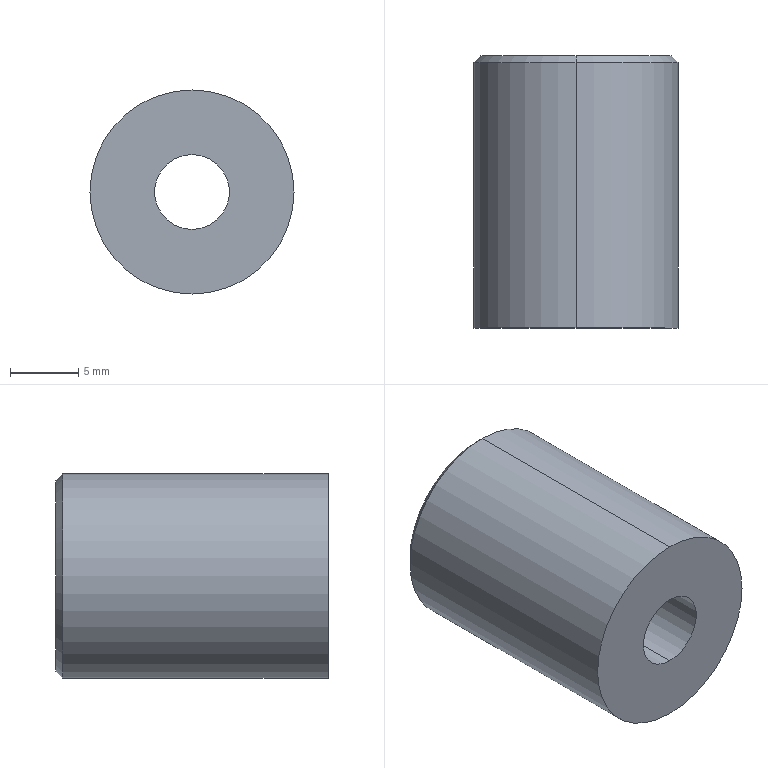Part | STEP file | PN_0011 | 1 solid | 11 faces | box 15 x 20 x 15 mm | volume 2655 mm3 | cylinder 6 | plane 3 | cone 2 | commonest cylinder face diameters 5.5 x2 9 x2 15 x2
STEP:
#1=CARTESIAN_POINT('',(0.,0.,0.));
#2=DIRECTION('',(0.,0.,1.));
#3=DIRECTION('',(1.,0.,0.));
#4=AXIS2_PLACEMENT_3D('',#1,#2,#3);
#5=CARTESIAN_POINT('',(0.,20.,7.));
#6=VERTEX_POINT('',#5);
#7=CARTESIAN_POINT('',(0.,20.,-7.));
#8=VERTEX_POINT('',#7);
#9=CARTESIAN_POINT('',(0.,20.,0.));
#10=DIRECTION('',(0.,1.,0.));
#11=DIRECTION('',(0.,0.,1.));
#12=AXIS2_PLACEMENT_3D('',#9,#10,#11);
#13=CIRCLE('',#12,7.);
#14=CARTESIAN_POINT('',(0.,20.,0.));
#15=DIRECTION('',(0.,-1.,0.));
#16=DIRECTION('',(0.,0.,-1.));
#17=AXIS2_PLACEMENT_3D('',#14,#15,#16);
#18=CONICAL_SURFACE('',#17,7.,0.7854);
#19=CARTESIAN_POINT('',(3.142,0.));
#20=DIRECTION('',(-1.,0.));
#21=VECTOR('',#20,1.);
#22=LINE('',#19,#21);
#23=(GEOMETRIC_REPRESENTATION_CONTEXT(2)PARAMETRIC_REPRESENTATION_CONTEXT()REPRESENTATION_CONTEXT('',''));
#24=DEFINITIONAL_REPRESENTATION('',(#22),#23);
#25=PCURVE('',#18,#24);
#26=CARTESIAN_POINT('',(0.,20.,0.));
#27=DIRECTION('',(0.,1.,0.));
#28=DIRECTION('',(0.,0.,1.));
#29=AXIS2_PLACEMENT_3D('',#26,#27,#28);
#30=PLANE('',#29);
#31=CARTESIAN_POINT('',(0.,0.));
#32=DIRECTION('',(1.,0.));
#33=AXIS2_PLACEMENT_2D('',#31,#32);
#34=CIRCLE('',#33,7.);
#35=(GEOMETRIC_REPRESENTATION_CONTEXT(2)PARAMETRIC_REPRESENTATION_CONTEXT()REPRESENTATION_CONTEXT('',''));
#36=DEFINITIONAL_REPRESENTATION('',(#34),#35);
#37=PCURVE('',#30,#36);
#38=SURFACE_CURVE('',#13,(#25,#37),.PCURVE_S1.);
#39=EDGE_CURVE('',#6,#8,#38,.T.);
#40=ORIENTED_EDGE('',*,*,#39,.F.);
#41=CARTESIAN_POINT('',(0.,19.5,7.5));
#42=VERTEX_POINT('',#41);
#43=CARTESIAN_POINT('',(0.,20.,7.));
#44=DIRECTION('',(0.,-0.7071,0.7071));
#45=VECTOR('',#44,1.);
#46=LINE('',#43,#45);
#47=CARTESIAN_POINT('',(3.142,0.));
#48=DIRECTION('',(0.,1.));
#49=VECTOR('',#48,1.);
#50=LINE('',#47,#49);
#51=(GEOMETRIC_REPRESENTATION_CONTEXT(2)PARAMETRIC_REPRESENTATION_CONTEXT()REPRESENTATION_CONTEXT('',''));
#52=DEFINITIONAL_REPRESENTATION('',(#50),#51);
#53=PCURVE('',#18,#52);
#54=CARTESIAN_POINT('',(0.,20.,0.));
#55=DIRECTION('',(0.,-1.,0.));
#56=DIRECTION('',(0.,0.,-1.));
#57=AXIS2_PLACEMENT_3D('',#54,#55,#56);
#58=CONICAL_SURFACE('',#57,7.,0.7854);
#59=CARTESIAN_POINT('',(3.142,0.));
#60=DIRECTION('',(0.,1.));
#61=VECTOR('',#60,1.);
#62=LINE('',#59,#61);
#63=(GEOMETRIC_REPRESENTATION_CONTEXT(2)PARAMETRIC_REPRESENTATION_CONTEXT()REPRESENTATION_CONTEXT('',''));
#64=DEFINITIONAL_REPRESENTATION('',(#62),#63);
#65=PCURVE('',#58,#64);
#66=SURFACE_CURVE('',#46,(#53,#65),.PCURVE_S1.);
#67=EDGE_CURVE('',#6,#42,#66,.T.);
#68=ORIENTED_EDGE('',*,*,#67,.T.);
#69=CARTESIAN_POINT('',(0.,19.5,-7.5));
#70=VERTEX_POINT('',#69);
#71=CARTESIAN_POINT('',(0.,19.5,0.));
#72=DIRECTION('',(0.,-1.,0.));
#73=DIRECTION('',(0.,0.,1.));
#74=AXIS2_PLACEMENT_3D('',#71,#72,#73);
#75=CIRCLE('',#74,7.5);
#76=CARTESIAN_POINT('',(-3.142,0.5));
#77=DIRECTION('',(1.,0.));
#78=VECTOR('',#77,1.);
#79=LINE('',#76,#78);
#80=(GEOMETRIC_REPRESENTATION_CONTEXT(2)PARAMETRIC_REPRESENTATION_CONTEXT()REPRESENTATION_CONTEXT('',''));
#81=DEFINITIONAL_REPRESENTATION('',(#79),#80);
#82=PCURVE('',#18,#81);
#83=CARTESIAN_POINT('',(0.,20.,0.));
#84=DIRECTION('',(0.,-1.,0.));
#85=DIRECTION('',(0.,0.,-1.));
#86=AXIS2_PLACEMENT_3D('',#83,#84,#85);
#87=CYLINDRICAL_SURFACE('',#86,7.5);
#88=CARTESIAN_POINT('',(-3.142,0.5));
#89=DIRECTION('',(1.,0.));
#90=VECTOR('',#89,1.);
#91=LINE('',#88,#90);
#92=(GEOMETRIC_REPRESENTATION_CONTEXT(2)PARAMETRIC_REPRESENTATION_CONTEXT()REPRESENTATION_CONTEXT('',''));
#93=DEFINITIONAL_REPRESENTATION('',(#91),#92);
#94=PCURVE('',#87,#93);
#95=SURFACE_CURVE('',#75,(#82,#94),.PCURVE_S1.);
#96=EDGE_CURVE('',#70,#42,#95,.T.);
#97=ORIENTED_EDGE('',*,*,#96,.F.);
#98=CARTESIAN_POINT('',(0.,20.,-7.));
#99=DIRECTION('',(0.,-0.7071,-0.7071));
#100=VECTOR('',#99,1.);
#101=LINE('',#98,#100);
#102=CARTESIAN_POINT('',(0.,0.));
#103=DIRECTION('',(0.,1.));
#104=VECTOR('',#103,1.);
#105=LINE('',#102,#104);
#106=(GEOMETRIC_REPRESENTATION_CONTEXT(2)PARAMETRIC_REPRESENTATION_CONTEXT()REPRESENTATION_CONTEXT('',''));
#107=DEFINITIONAL_REPRESENTATION('',(#105),#106);
#108=PCURVE('',#18,#107);
#109=CARTESIAN_POINT('',(6.283,0.));
#110=DIRECTION('',(0.,1.));
#111=VECTOR('',#110,1.);
#112=LINE('',#109,#111);
#113=(GEOMETRIC_REPRESENTATION_CONTEXT(2)PARAMETRIC_REPRESENTATION_CONTEXT()REPRESENTATION_CONTEXT('',''));
#114=DEFINITIONAL_REPRESENTATION('',(#112),#113);
#115=PCURVE('',#58,#114);
#116=SURFACE_CURVE('',#101,(#108,#115),.PCURVE_S1.);
#117=EDGE_CURVE('',#8,#70,#116,.T.);
#118=ORIENTED_EDGE('',*,*,#117,.F.);
#119=EDGE_LOOP('',(#40,#68,#97,#118));
#120=FACE_BOUND('',#119,.T.);
#121=ADVANCED_FACE('',(#120),#18,.T.);
#122=CARTESIAN_POINT('',(0.,10.,4.5));
#123=VERTEX_POINT('',#122);
#124=CARTESIAN_POINT('',(0.,20.,4.5));
#125=VERTEX_POINT('',#124);
#126=CARTESIAN_POINT('',(0.,20.,4.5));
#127=DIRECTION('',(0.,1.,0.));
#128=VECTOR('',#127,1.);
#129=LINE('',#126,#128);
#130=CARTESIAN_POINT('',(0.,20.,0.));
#131=DIRECTION('',(0.,1.,0.));
#132=DIRECTION('',(0.,0.,1.));
#133=AXIS2_PLACEMENT_3D('',#130,#131,#132);
#134=CYLINDRICAL_SURFACE('',#133,4.5);
#135=CARTESIAN_POINT('',(6.283,0.));
#136=DIRECTION('',(0.,1.));
#137=VECTOR('',#136,1.);
#138=LINE('',#135,#137);
#139=(GEOMETRIC_REPRESENTATION_CONTEXT(2)PARAMETRIC_REPRESENTATION_CONTEXT()REPRESENTATION_CONTEXT('',''));
#140=DEFINITIONAL_REPRESENTATION('',(#138),#139);
#141=PCURVE('',#134,#140);
#142=CARTESIAN_POINT('',(0.,20.,0.));
#143=DIRECTION('',(0.,1.,0.));
#144=DIRECTION('',(0.,0.,1.));
#145=AXIS2_PLACEMENT_3D('',#142,#143,#144);
#146=CYLINDRICAL_SURFACE('',#145,4.5);
#147=CARTESIAN_POINT('',(0.,0.));
#148=DIRECTION('',(0.,1.));
#149=VECTOR('',#148,1.);
#150=LINE('',#147,#149);
#151=(GEOMETRIC_REPRESENTATION_CONTEXT(2)PARAMETRIC_REPRESENTATION_CONTEXT()REPRESENTATION_CONTEXT('',''));
#152=DEFINITIONAL_REPRESENTATION('',(#150),#151);
#153=PCURVE('',#146,#152);
#154=SURFACE_CURVE('',#129,(#141,#153),.PCURVE_S1.);
#155=EDGE_CURVE('',#123,#125,#154,.T.);
#156=ORIENTED_EDGE('',*,*,#155,.T.);
#157=CARTESIAN_POINT('',(0.,20.,-4.5));
#158=VERTEX_POINT('',#157);
#159=CARTESIAN_POINT('',(0.,20.,0.));
#160=DIRECTION('',(0.,1.,0.));
#161=DIRECTION('',(0.,0.,1.));
#162=AXIS2_PLACEMENT_3D('',#159,#160,#161);
#163=CIRCLE('',#162,4.5);
#164=CARTESIAN_POINT('',(0.,0.));
#165=DIRECTION('',(1.,0.));
#166=VECTOR('',#165,1.);
#167=LINE('',#164,#166);
#168=(GEOMETRIC_REPRESENTATION_CONTEXT(2)PARAMETRIC_REPRESENTATION_CONTEXT()REPRESENTATION_CONTEXT('',''));
#169=DEFINITIONAL_REPRESENTATION('',(#167),#168);
#170=PCURVE('',#134,#169);
#171=CARTESIAN_POINT('',(0.,0.));
#172=DIRECTION('',(1.,0.));
#173=AXIS2_PLACEMENT_2D('',#171,#172);
#174=CIRCLE('',#173,4.5);
#175=(GEOMETRIC_REPRESENTATION_CONTEXT(2)PARAMETRIC_REPRESENTATION_CONTEXT()REPRESENTATION_CONTEXT('',''));
#176=DEFINITIONAL_REPRESENTATION('',(#174),#175);
#177=PCURVE('',#30,#176);
#178=SURFACE_CURVE('',#163,(#170,#177),.PCURVE_S1.);
#179=EDGE_CURVE('',#158,#125,#178,.T.);
#180=ORIENTED_EDGE('',*,*,#179,.F.);
#181=CARTESIAN_POINT('',(0.,10.,-4.5));
#182=VERTEX_POINT('',#181);
#183=CARTESIAN_POINT('',(0.,20.,-4.5));
#184=DIRECTION('',(0.,1.,0.));
#185=VECTOR('',#184,1.);
#186=LINE('',#183,#185);
#187=CARTESIAN_POINT('',(3.142,0.));
#188=DIRECTION('',(0.,1.));
#189=VECTOR('',#188,1.);
#190=LINE('',#187,#189);
#191=(GEOMETRIC_REPRESENTATION_CONTEXT(2)PARAMETRIC_REPRESENTATION_CONTEXT()REPRESENTATION_CONTEXT('',''));
#192=DEFINITIONAL_REPRESENTATION('',(#190),#191);
#193=PCURVE('',#134,#192);
#194=CARTESIAN_POINT('',(3.142,0.));
#195=DIRECTION('',(0.,1.));
#196=VECTOR('',#195,1.);
#197=LINE('',#194,#196);
#198=(GEOMETRIC_REPRESENTATION_CONTEXT(2)PARAMETRIC_REPRESENTATION_CONTEXT()REPRESENTATION_CONTEXT('',''));
#199=DEFINITIONAL_REPRESENTATION('',(#197),#198);
#200=PCURVE('',#146,#199);
#201=SURFACE_CURVE('',#186,(#193,#200),.PCURVE_S1.);
#202=EDGE_CURVE('',#182,#158,#201,.T.);
#203=ORIENTED_EDGE('',*,*,#202,.F.);
#204=CARTESIAN_POINT('',(0.,10.,0.));
#205=DIRECTION('',(0.,1.,0.));
#206=DIRECTION('',(0.,0.,1.));
#207=AXIS2_PLACEMENT_3D('',#204,#205,#206);
#208=CIRCLE('',#207,4.5);
#209=CARTESIAN_POINT('',(0.,-10.));
#210=DIRECTION('',(1.,0.));
#211=VECTOR('',#210,1.);
#212=LINE('',#209,#211);
#213=(GEOMETRIC_REPRESENTATION_CONTEXT(2)PARAMETRIC_REPRESENTATION_CONTEXT()REPRESENTATION_CONTEXT('',''));
#214=DEFINITIONAL_REPRESENTATION('',(#212),#213);
#215=PCURVE('',#134,#214);
#216=CARTESIAN_POINT('',(2.75,10.,0.));
#217=DIRECTION('',(0.,-1.,0.));
#218=DIRECTION('',(0.,0.,-1.));
#219=AXIS2_PLACEMENT_3D('',#216,#217,#218);
#220=PLANE('',#219);
#221=CARTESIAN_POINT('',(-4.5,-2.75));
#222=CARTESIAN_POINT('',(-4.5,5.044));
#223=CARTESIAN_POINT('',(2.25,1.147));
#224=CARTESIAN_POINT('',(9.,-2.75));
#225=CARTESIAN_POINT('',(2.25,-6.647));
#226=CARTESIAN_POINT('',(-4.5,-10.544));
#227=CARTESIAN_POINT('',(-4.5,-2.75));
#228=(BOUNDED_CURVE()B_SPLINE_CURVE(2,(#221,#222,#223,#224,#225,#226,#227),.UNSPECIFIED.,.T.,.F.)B_SPLINE_CURVE_WITH_KNOTS((1,2,2,2,2,1),(-2.094,0.,2.094,4.189,6.283,8.378),.UNSPECIFIED.)CURVE()GEOMETRIC_REPRESENTATION_ITEM()RATIONAL_B_SPLINE_CURVE((1.,0.5,1.,0.5,1.,0.5,1.))REPRESENTATION_ITEM(''));
#229=(GEOMETRIC_REPRESENTATION_CONTEXT(2)PARAMETRIC_REPRESENTATION_CONTEXT()REPRESENTATION_CONTEXT('',''));
#230=DEFINITIONAL_REPRESENTATION('',(#228),#229);
#231=PCURVE('',#220,#230);
#232=SURFACE_CURVE('',#208,(#215,#231),.PCURVE_S1.);
#233=EDGE_CURVE('',#182,#123,#232,.T.);
#234=ORIENTED_EDGE('',*,*,#233,.T.);
#235=EDGE_LOOP('',(#156,#180,#203,#234));
#236=FACE_BOUND('',#235,.F.);
#237=ADVANCED_FACE('',(#236),#134,.F.);
#238=CARTESIAN_POINT('',(0.,0.,2.75));
#239=VERTEX_POINT('',#238);
#240=CARTESIAN_POINT('',(0.,10.,2.75));
#241=VERTEX_POINT('',#240);
#242=CARTESIAN_POINT('',(0.,20.,2.75));
#243=DIRECTION('',(0.,1.,0.));
#244=VECTOR('',#243,1.);
#245=LINE('',#242,#244);
#246=CARTESIAN_POINT('',(0.,20.,0.));
#247=DIRECTION('',(0.,1.,0.));
#248=DIRECTION('',(0.,0.,1.));
#249=AXIS2_PLACEMENT_3D('',#246,#247,#248);
#250=CYLINDRICAL_SURFACE('',#249,2.75);
#251=CARTESIAN_POINT('',(6.283,0.));
#252=DIRECTION('',(0.,1.));
#253=VECTOR('',#252,1.);
#254=LINE('',#251,#253);
#255=(GEOMETRIC_REPRESENTATION_CONTEXT(2)PARAMETRIC_REPRESENTATION_CONTEXT()REPRESENTATION_CONTEXT('',''));
#256=DEFINITIONAL_REPRESENTATION('',(#254),#255);
#257=PCURVE('',#250,#256);
#258=CARTESIAN_POINT('',(0.,20.,0.));
#259=DIRECTION('',(0.,1.,0.));
#260=DIRECTION('',(0.,0.,1.));
#261=AXIS2_PLACEMENT_3D('',#258,#259,#260);
#262=CYLINDRICAL_SURFACE('',#261,2.75);
#263=CARTESIAN_POINT('',(0.,0.));
#264=DIRECTION('',(0.,1.));
#265=VECTOR('',#264,1.);
#266=LINE('',#263,#265);
#267=(GEOMETRIC_REPRESENTATION_CONTEXT(2)PARAMETRIC_REPRESENTATION_CONTEXT()REPRESENTATION_CONTEXT('',''));
#268=DEFINITIONAL_REPRESENTATION('',(#266),#267);
#269=PCURVE('',#262,#268);
#270=SURFACE_CURVE('',#245,(#257,#269),.PCURVE_S1.);
#271=EDGE_CURVE('',#239,#241,#270,.T.);
#272=ORIENTED_EDGE('',*,*,#271,.T.);
#273=CARTESIAN_POINT('',(0.,10.,-2.75));
#274=VERTEX_POINT('',#273);
#275=CARTESIAN_POINT('',(0.,10.,0.));
#276=DIRECTION('',(0.,1.,0.));
#277=DIRECTION('',(0.,0.,1.));
#278=AXIS2_PLACEMENT_3D('',#275,#276,#277);
#279=CIRCLE('',#278,2.75);
#280=CARTESIAN_POINT('',(0.,-10.));
#281=DIRECTION('',(1.,0.));
#282=VECTOR('',#281,1.);
#283=LINE('',#280,#282);
#284=(GEOMETRIC_REPRESENTATION_CONTEXT(2)PARAMETRIC_REPRESENTATION_CONTEXT()REPRESENTATION_CONTEXT('',''));
#285=DEFINITIONAL_REPRESENTATION('',(#283),#284);
#286=PCURVE('',#250,#285);
#287=CARTESIAN_POINT('',(-2.75,-2.75));
#288=CARTESIAN_POINT('',(-2.75,2.013));
#289=CARTESIAN_POINT('',(1.375,-0.3684));
#290=CARTESIAN_POINT('',(5.5,-2.75));
#291=CARTESIAN_POINT('',(1.375,-5.132));
#292=CARTESIAN_POINT('',(-2.75,-7.513));
#293=CARTESIAN_POINT('',(-2.75,-2.75));
#294=(BOUNDED_CURVE()B_SPLINE_CURVE(2,(#287,#288,#289,#290,#291,#292,#293),.UNSPECIFIED.,.T.,.F.)B_SPLINE_CURVE_WITH_KNOTS((1,2,2,2,2,1),(-2.094,0.,2.094,4.189,6.283,8.378),.UNSPECIFIED.)CURVE()GEOMETRIC_REPRESENTATION_ITEM()RATIONAL_B_SPLINE_CURVE((1.,0.5,1.,0.5,1.,0.5,1.))REPRESENTATION_ITEM(''));
#295=(GEOMETRIC_REPRESENTATION_CONTEXT(2)PARAMETRIC_REPRESENTATION_CONTEXT()REPRESENTATION_CONTEXT('',''));
#296=DEFINITIONAL_REPRESENTATION('',(#294),#295);
#297=PCURVE('',#220,#296);
#298=SURFACE_CURVE('',#279,(#286,#297),.PCURVE_S1.);
#299=EDGE_CURVE('',#274,#241,#298,.T.);
#300=ORIENTED_EDGE('',*,*,#299,.F.);
#301=CARTESIAN_POINT('',(0.,0.,-2.75));
#302=VERTEX_POINT('',#301);
#303=CARTESIAN_POINT('',(0.,20.,-2.75));
#304=DIRECTION('',(0.,1.,0.));
#305=VECTOR('',#304,1.);
#306=LINE('',#303,#305);
#307=CARTESIAN_POINT('',(3.142,0.));
#308=DIRECTION('',(0.,1.));
#309=VECTOR('',#308,1.);
#310=LINE('',#307,#309);
#311=(GEOMETRIC_REPRESENTATION_CONTEXT(2)PARAMETRIC_REPRESENTATION_CONTEXT()REPRESENTATION_CONTEXT('',''));
#312=DEFINITIONAL_REPRESENTATION('',(#310),#311);
#313=PCURVE('',#250,#312);
#314=CARTESIAN_POINT('',(3.142,0.));
#315=DIRECTION('',(0.,1.));
#316=VECTOR('',#315,1.);
#317=LINE('',#314,#316);
#318=(GEOMETRIC_REPRESENTATION_CONTEXT(2)PARAMETRIC_REPRESENTATION_CONTEXT()REPRESENTATION_CONTEXT('',''));
#319=DEFINITIONAL_REPRESENTATION('',(#317),#318);
#320=PCURVE('',#262,#319);
#321=SURFACE_CURVE('',#306,(#313,#320),.PCURVE_S1.);
#322=EDGE_CURVE('',#302,#274,#321,.T.);
#323=ORIENTED_EDGE('',*,*,#322,.F.);
#324=CARTESIAN_POINT('',(0.,0.,0.));
#325=DIRECTION('',(0.,1.,0.));
#326=DIRECTION('',(0.,0.,1.));
#327=AXIS2_PLACEMENT_3D('',#324,#325,#326);
#328=CIRCLE('',#327,2.75);
#329=CARTESIAN_POINT('',(0.,-20.));
#330=DIRECTION('',(1.,0.));
#331=VECTOR('',#330,1.);
#332=LINE('',#329,#331);
#333=(GEOMETRIC_REPRESENTATION_CONTEXT(2)PARAMETRIC_REPRESENTATION_CONTEXT()REPRESENTATION_CONTEXT('',''));
#334=DEFINITIONAL_REPRESENTATION('',(#332),#333);
#335=PCURVE('',#250,#334);
#336=CARTESIAN_POINT('',(0.,0.,0.));
#337=DIRECTION('',(0.,1.,0.));
#338=DIRECTION('',(0.,0.,1.));
#339=AXIS2_PLACEMENT_3D('',#336,#337,#338);
#340=PLANE('',#339);
#341=CARTESIAN_POINT('',(0.,0.));
#342=DIRECTION('',(1.,0.));
#343=AXIS2_PLACEMENT_2D('',#341,#342);
#344=CIRCLE('',#343,2.75);
#345=(GEOMETRIC_REPRESENTATION_CONTEXT(2)PARAMETRIC_REPRESENTATION_CONTEXT()REPRESENTATION_CONTEXT('',''));
#346=DEFINITIONAL_REPRESENTATION('',(#344),#345);
#347=PCURVE('',#340,#346);
#348=SURFACE_CURVE('',#328,(#335,#347),.PCURVE_S1.);
#349=EDGE_CURVE('',#302,#239,#348,.T.);
#350=ORIENTED_EDGE('',*,*,#349,.T.);
#351=EDGE_LOOP('',(#272,#300,#323,#350));
#352=FACE_BOUND('',#351,.F.);
#353=ADVANCED_FACE('',(#352),#250,.F.);
#354=ORIENTED_EDGE('',*,*,#96,.T.);
#355=CARTESIAN_POINT('',(0.,0.,7.5));
#356=VERTEX_POINT('',#355);
#357=CARTESIAN_POINT('',(0.,20.,7.5));
#358=DIRECTION('',(0.,-1.,0.));
#359=VECTOR('',#358,1.);
#360=LINE('',#357,#359);
#361=CARTESIAN_POINT('',(3.142,0.));
#362=DIRECTION('',(0.,1.));
#363=VECTOR('',#362,1.);
#364=LINE('',#361,#363);
#365=(GEOMETRIC_REPRESENTATION_CONTEXT(2)PARAMETRIC_REPRESENTATION_CONTEXT()REPRESENTATION_CONTEXT('',''));
#366=DEFINITIONAL_REPRESENTATION('',(#364),#365);
#367=PCURVE('',#87,#366);
#368=CARTESIAN_POINT('',(0.,20.,0.));
#369=DIRECTION('',(0.,-1.,0.));
#370=DIRECTION('',(0.,0.,-1.));
#371=AXIS2_PLACEMENT_3D('',#368,#369,#370);
#372=CYLINDRICAL_SURFACE('',#371,7.5);
#373=CARTESIAN_POINT('',(3.142,0.));
#374=DIRECTION('',(0.,1.));
#375=VECTOR('',#374,1.);
#376=LINE('',#373,#375);
#377=(GEOMETRIC_REPRESENTATION_CONTEXT(2)PARAMETRIC_REPRESENTATION_CONTEXT()REPRESENTATION_CONTEXT('',''));
#378=DEFINITIONAL_REPRESENTATION('',(#376),#377);
#379=PCURVE('',#372,#378);
#380=SURFACE_CURVE('',#360,(#367,#379),.PCURVE_S1.);
#381=EDGE_CURVE('',#42,#356,#380,.T.);
#382=ORIENTED_EDGE('',*,*,#381,.T.);
#383=CARTESIAN_POINT('',(0.,0.,-7.5));
#384=VERTEX_POINT('',#383);
#385=CARTESIAN_POINT('',(0.,0.,0.));
#386=DIRECTION('',(0.,1.,0.));
#387=DIRECTION('',(0.,0.,1.));
#388=AXIS2_PLACEMENT_3D('',#385,#386,#387);
#389=CIRCLE('',#388,7.5);
#390=CARTESIAN_POINT('',(3.142,20.));
#391=DIRECTION('',(-1.,0.));
#392=VECTOR('',#391,1.);
#393=LINE('',#390,#392);
#394=(GEOMETRIC_REPRESENTATION_CONTEXT(2)PARAMETRIC_REPRESENTATION_CONTEXT()REPRESENTATION_CONTEXT('',''));
#395=DEFINITIONAL_REPRESENTATION('',(#393),#394);
#396=PCURVE('',#87,#395);
#397=CARTESIAN_POINT('',(0.,0.));
#398=DIRECTION('',(1.,0.));
#399=AXIS2_PLACEMENT_2D('',#397,#398);
#400=CIRCLE('',#399,7.5);
#401=(GEOMETRIC_REPRESENTATION_CONTEXT(2)PARAMETRIC_REPRESENTATION_CONTEXT()REPRESENTATION_CONTEXT('',''));
#402=DEFINITIONAL_REPRESENTATION('',(#400),#401);
#403=PCURVE('',#340,#402);
#404=SURFACE_CURVE('',#389,(#396,#403),.PCURVE_S1.);
#405=EDGE_CURVE('',#356,#384,#404,.T.);
#406=ORIENTED_EDGE('',*,*,#405,.T.);
#407=CARTESIAN_POINT('',(0.,20.,-7.5));
#408=DIRECTION('',(0.,-1.,0.));
#409=VECTOR('',#408,1.);
#410=LINE('',#407,#409);
#411=CARTESIAN_POINT('',(0.,0.));
#412=DIRECTION('',(0.,1.));
#413=VECTOR('',#412,1.);
#414=LINE('',#411,#413);
#415=(GEOMETRIC_REPRESENTATION_CONTEXT(2)PARAMETRIC_REPRESENTATION_CONTEXT()REPRESENTATION_CONTEXT('',''));
#416=DEFINITIONAL_REPRESENTATION('',(#414),#415);
#417=PCURVE('',#87,#416);
#418=CARTESIAN_POINT('',(6.283,0.));
#419=DIRECTION('',(0.,1.));
#420=VECTOR('',#419,1.);
#421=LINE('',#418,#420);
#422=(GEOMETRIC_REPRESENTATION_CONTEXT(2)PARAMETRIC_REPRESENTATION_CONTEXT()REPRESENTATION_CONTEXT('',''));
#423=DEFINITIONAL_REPRESENTATION('',(#421),#422);
#424=PCURVE('',#372,#423);
#425=SURFACE_CURVE('',#410,(#417,#424),.PCURVE_S1.);
#426=EDGE_CURVE('',#70,#384,#425,.T.);
#427=ORIENTED_EDGE('',*,*,#426,.F.);
#428=EDGE_LOOP('',(#354,#382,#406,#427));
#429=FACE_BOUND('',#428,.T.);
#430=ADVANCED_FACE('',(#429),#87,.T.);
#431=ORIENTED_EDGE('',*,*,#381,.F.);
#432=CARTESIAN_POINT('',(0.,19.5,0.));
#433=DIRECTION('',(0.,-1.,0.));
#434=DIRECTION('',(0.,0.,1.));
#435=AXIS2_PLACEMENT_3D('',#432,#433,#434);
#436=CIRCLE('',#435,7.5);
#437=CARTESIAN_POINT('',(3.142,0.5));
#438=DIRECTION('',(1.,0.));
#439=VECTOR('',#438,1.);
#440=LINE('',#437,#439);
#441=(GEOMETRIC_REPRESENTATION_CONTEXT(2)PARAMETRIC_REPRESENTATION_CONTEXT()REPRESENTATION_CONTEXT('',''));
#442=DEFINITIONAL_REPRESENTATION('',(#440),#441);
#443=PCURVE('',#372,#442);
#444=CARTESIAN_POINT('',(3.142,0.5));
#445=DIRECTION('',(1.,0.));
#446=VECTOR('',#445,1.);
#447=LINE('',#444,#446);
#448=(GEOMETRIC_REPRESENTATION_CONTEXT(2)PARAMETRIC_REPRESENTATION_CONTEXT()REPRESENTATION_CONTEXT('',''));
#449=DEFINITIONAL_REPRESENTATION('',(#447),#448);
#450=PCURVE('',#58,#449);
#451=SURFACE_CURVE('',#436,(#443,#450),.PCURVE_S1.);
#452=EDGE_CURVE('',#42,#70,#451,.T.);
#453=ORIENTED_EDGE('',*,*,#452,.T.);
#454=ORIENTED_EDGE('',*,*,#426,.T.);
#455=CARTESIAN_POINT('',(0.,0.,0.));
#456=DIRECTION('',(0.,1.,0.));
#457=DIRECTION('',(0.,0.,1.));
#458=AXIS2_PLACEMENT_3D('',#455,#456,#457);
#459=CIRCLE('',#458,7.5);
#460=CARTESIAN_POINT('',(9.425,20.));
#461=DIRECTION('',(-1.,0.));
#462=VECTOR('',#461,1.);
#463=LINE('',#460,#462);
#464=(GEOMETRIC_REPRESENTATION_CONTEXT(2)PARAMETRIC_REPRESENTATION_CONTEXT()REPRESENTATION_CONTEXT('',''));
#465=DEFINITIONAL_REPRESENTATION('',(#463),#464);
#466=PCURVE('',#372,#465);
#467=CARTESIAN_POINT('',(0.,0.));
#468=DIRECTION('',(1.,0.));
#469=AXIS2_PLACEMENT_2D('',#467,#468);
#470=CIRCLE('',#469,7.5);
#471=(GEOMETRIC_REPRESENTATION_CONTEXT(2)PARAMETRIC_REPRESENTATION_CONTEXT()REPRESENTATION_CONTEXT('',''));
#472=DEFINITIONAL_REPRESENTATION('',(#470),#471);
#473=PCURVE('',#340,#472);
#474=SURFACE_CURVE('',#459,(#466,#473),.PCURVE_S1.);
#475=EDGE_CURVE('',#384,#356,#474,.T.);
#476=ORIENTED_EDGE('',*,*,#475,.T.);
#477=EDGE_LOOP('',(#431,#453,#454,#476));
#478=FACE_BOUND('',#477,.T.);
#479=ADVANCED_FACE('',(#478),#372,.T.);
#480=CARTESIAN_POINT('',(0.,20.,0.));
#481=DIRECTION('',(0.,1.,0.));
#482=DIRECTION('',(0.,0.,1.));
#483=AXIS2_PLACEMENT_3D('',#480,#481,#482);
#484=CIRCLE('',#483,7.);
#485=CARTESIAN_POINT('',(0.,0.));
#486=DIRECTION('',(1.,0.));
#487=AXIS2_PLACEMENT_2D('',#485,#486);
#488=CIRCLE('',#487,7.);
#489=(GEOMETRIC_REPRESENTATION_CONTEXT(2)PARAMETRIC_REPRESENTATION_CONTEXT()REPRESENTATION_CONTEXT('',''));
#490=DEFINITIONAL_REPRESENTATION('',(#488),#489);
#491=PCURVE('',#30,#490);
#492=CARTESIAN_POINT('',(9.425,0.));
#493=DIRECTION('',(-1.,0.));
#494=VECTOR('',#493,1.);
#495=LINE('',#492,#494);
#496=(GEOMETRIC_REPRESENTATION_CONTEXT(2)PARAMETRIC_REPRESENTATION_CONTEXT()REPRESENTATION_CONTEXT('',''));
#497=DEFINITIONAL_REPRESENTATION('',(#495),#496);
#498=PCURVE('',#58,#497);
#499=SURFACE_CURVE('',#484,(#491,#498),.PCURVE_S1.);
#500=EDGE_CURVE('',#8,#6,#499,.T.);
#501=ORIENTED_EDGE('',*,*,#500,.T.);
#502=ORIENTED_EDGE('',*,*,#39,.T.);
#503=EDGE_LOOP('',(#501,#502));
#504=FACE_BOUND('',#503,.T.);
#505=CARTESIAN_POINT('',(0.,20.,0.));
#506=DIRECTION('',(0.,1.,0.));
#507=DIRECTION('',(0.,0.,1.));
#508=AXIS2_PLACEMENT_3D('',#505,#506,#507);
#509=CIRCLE('',#508,4.5);
#510=CARTESIAN_POINT('',(0.,0.));
#511=DIRECTION('',(1.,0.));
#512=AXIS2_PLACEMENT_2D('',#510,#511);
#513=CIRCLE('',#512,4.5);
#514=(GEOMETRIC_REPRESENTATION_CONTEXT(2)PARAMETRIC_REPRESENTATION_CONTEXT()REPRESENTATION_CONTEXT('',''));
#515=DEFINITIONAL_REPRESENTATION('',(#513),#514);
#516=PCURVE('',#30,#515);
#517=CARTESIAN_POINT('',(0.,0.));
#518=DIRECTION('',(1.,0.));
#519=VECTOR('',#518,1.);
#520=LINE('',#517,#519);
#521=(GEOMETRIC_REPRESENTATION_CONTEXT(2)PARAMETRIC_REPRESENTATION_CONTEXT()REPRESENTATION_CONTEXT('',''));
#522=DEFINITIONAL_REPRESENTATION('',(#520),#521);
#523=PCURVE('',#146,#522);
#524=SURFACE_CURVE('',#509,(#516,#523),.PCURVE_S1.);
#525=EDGE_CURVE('',#125,#158,#524,.T.);
#526=ORIENTED_EDGE('',*,*,#525,.F.);
#527=ORIENTED_EDGE('',*,*,#179,.F.);
#528=EDGE_LOOP('',(#526,#527));
#529=FACE_BOUND('',#528,.T.);
#530=ADVANCED_FACE('',(#504,#529),#30,.T.);
#531=CARTESIAN_POINT('',(0.,0.,0.));
#532=DIRECTION('',(0.,1.,0.));
#533=DIRECTION('',(0.,0.,1.));
#534=AXIS2_PLACEMENT_3D('',#531,#532,#533);
#535=CIRCLE('',#534,2.75);
#536=CARTESIAN_POINT('',(0.,0.));
#537=DIRECTION('',(1.,0.));
#538=AXIS2_PLACEMENT_2D('',#536,#537);
#539=CIRCLE('',#538,2.75);
#540=(GEOMETRIC_REPRESENTATION_CONTEXT(2)PARAMETRIC_REPRESENTATION_CONTEXT()REPRESENTATION_CONTEXT('',''));
#541=DEFINITIONAL_REPRESENTATION('',(#539),#540);
#542=PCURVE('',#340,#541);
#543=CARTESIAN_POINT('',(0.,-20.));
#544=DIRECTION('',(1.,0.));
#545=VECTOR('',#544,1.);
#546=LINE('',#543,#545);
#547=(GEOMETRIC_REPRESENTATION_CONTEXT(2)PARAMETRIC_REPRESENTATION_CONTEXT()REPRESENTATION_CONTEXT('',''));
#548=DEFINITIONAL_REPRESENTATION('',(#546),#547);
#549=PCURVE('',#262,#548);
#550=SURFACE_CURVE('',#535,(#542,#549),.PCURVE_S1.);
#551=EDGE_CURVE('',#239,#302,#550,.T.);
#552=ORIENTED_EDGE('',*,*,#551,.T.);
#553=ORIENTED_EDGE('',*,*,#349,.T.);
#554=EDGE_LOOP('',(#552,#553));
#555=FACE_BOUND('',#554,.T.);
#556=ORIENTED_EDGE('',*,*,#475,.F.);
#557=ORIENTED_EDGE('',*,*,#405,.F.);
#558=EDGE_LOOP('',(#556,#557));
#559=FACE_BOUND('',#558,.T.);
#560=ADVANCED_FACE('',(#555,#559),#340,.F.);
#561=CARTESIAN_POINT('',(0.,10.,0.));
#562=DIRECTION('',(0.,1.,0.));
#563=DIRECTION('',(0.,0.,1.));
#564=AXIS2_PLACEMENT_3D('',#561,#562,#563);
#565=CIRCLE('',#564,2.75);
#566=CARTESIAN_POINT('',(0.,-10.));
#567=DIRECTION('',(1.,0.));
#568=VECTOR('',#567,1.);
#569=LINE('',#566,#568);
#570=(GEOMETRIC_REPRESENTATION_CONTEXT(2)PARAMETRIC_REPRESENTATION_CONTEXT()REPRESENTATION_CONTEXT('',''));
#571=DEFINITIONAL_REPRESENTATION('',(#569),#570);
#572=PCURVE('',#262,#571);
#573=CARTESIAN_POINT('',(-2.75,-2.75));
#574=CARTESIAN_POINT('',(-2.75,2.013));
#575=CARTESIAN_POINT('',(1.375,-0.3684));
#576=CARTESIAN_POINT('',(5.5,-2.75));
#577=CARTESIAN_POINT('',(1.375,-5.132));
#578=CARTESIAN_POINT('',(-2.75,-7.513));
#579=CARTESIAN_POINT('',(-2.75,-2.75));
#580=(BOUNDED_CURVE()B_SPLINE_CURVE(2,(#573,#574,#575,#576,#577,#578,#579),.UNSPECIFIED.,.T.,.F.)B_SPLINE_CURVE_WITH_KNOTS((1,2,2,2,2,1),(-2.094,0.,2.094,4.189,6.283,8.378),.UNSPECIFIED.)CURVE()GEOMETRIC_REPRESENTATION_ITEM()RATIONAL_B_SPLINE_CURVE((1.,0.5,1.,0.5,1.,0.5,1.))REPRESENTATION_ITEM(''));
#581=(GEOMETRIC_REPRESENTATION_CONTEXT(2)PARAMETRIC_REPRESENTATION_CONTEXT()REPRESENTATION_CONTEXT('',''));
#582=DEFINITIONAL_REPRESENTATION('',(#580),#581);
#583=PCURVE('',#220,#582);
#584=SURFACE_CURVE('',#565,(#572,#583),.PCURVE_S1.);
#585=EDGE_CURVE('',#241,#274,#584,.T.);
#586=ORIENTED_EDGE('',*,*,#585,.F.);
#587=ORIENTED_EDGE('',*,*,#271,.F.);
#588=ORIENTED_EDGE('',*,*,#551,.T.);
#589=ORIENTED_EDGE('',*,*,#322,.T.);
#590=EDGE_LOOP('',(#586,#587,#588,#589));
#591=FACE_BOUND('',#590,.F.);
#592=ADVANCED_FACE('',(#591),#262,.F.);
#593=ORIENTED_EDGE('',*,*,#585,.F.);
#594=ORIENTED_EDGE('',*,*,#299,.F.);
#595=EDGE_LOOP('',(#593,#594));
#596=FACE_BOUND('',#595,.T.);
#597=CARTESIAN_POINT('',(0.,10.,0.));
#598=DIRECTION('',(0.,1.,0.));
#599=DIRECTION('',(0.,0.,1.));
#600=AXIS2_PLACEMENT_3D('',#597,#598,#599);
#601=CIRCLE('',#600,4.5);
#602=CARTESIAN_POINT('',(-4.5,-2.75));
#603=CARTESIAN_POINT('',(-4.5,5.044));
#604=CARTESIAN_POINT('',(2.25,1.147));
#605=CARTESIAN_POINT('',(9.,-2.75));
#606=CARTESIAN_POINT('',(2.25,-6.647));
#607=CARTESIAN_POINT('',(-4.5,-10.544));
#608=CARTESIAN_POINT('',(-4.5,-2.75));
#609=(BOUNDED_CURVE()B_SPLINE_CURVE(2,(#602,#603,#604,#605,#606,#607,#608),.UNSPECIFIED.,.T.,.F.)B_SPLINE_CURVE_WITH_KNOTS((1,2,2,2,2,1),(-2.094,0.,2.094,4.189,6.283,8.378),.UNSPECIFIED.)CURVE()GEOMETRIC_REPRESENTATION_ITEM()RATIONAL_B_SPLINE_CURVE((1.,0.5,1.,0.5,1.,0.5,1.))REPRESENTATION_ITEM(''));
#610=(GEOMETRIC_REPRESENTATION_CONTEXT(2)PARAMETRIC_REPRESENTATION_CONTEXT()REPRESENTATION_CONTEXT('',''));
#611=DEFINITIONAL_REPRESENTATION('',(#609),#610);
#612=PCURVE('',#220,#611);
#613=CARTESIAN_POINT('',(0.,-10.));
#614=DIRECTION('',(1.,0.));
#615=VECTOR('',#614,1.);
#616=LINE('',#613,#615);
#617=(GEOMETRIC_REPRESENTATION_CONTEXT(2)PARAMETRIC_REPRESENTATION_CONTEXT()REPRESENTATION_CONTEXT('',''));
#618=DEFINITIONAL_REPRESENTATION('',(#616),#617);
#619=PCURVE('',#146,#618);
#620=SURFACE_CURVE('',#601,(#612,#619),.PCURVE_S1.);
#621=EDGE_CURVE('',#123,#182,#620,.T.);
#622=ORIENTED_EDGE('',*,*,#621,.T.);
#623=ORIENTED_EDGE('',*,*,#233,.T.);
#624=EDGE_LOOP('',(#622,#623));
#625=FACE_BOUND('',#624,.T.);
#626=ADVANCED_FACE('',(#596,#625),#220,.F.);
#627=ORIENTED_EDGE('',*,*,#525,.F.);
#628=ORIENTED_EDGE('',*,*,#155,.F.);
#629=ORIENTED_EDGE('',*,*,#621,.T.);
#630=ORIENTED_EDGE('',*,*,#202,.T.);
#631=EDGE_LOOP('',(#627,#628,#629,#630));
#632=FACE_BOUND('',#631,.F.);
#633=ADVANCED_FACE('',(#632),#146,.F.);
#634=ORIENTED_EDGE('',*,*,#67,.F.);
#635=ORIENTED_EDGE('',*,*,#500,.F.);
#636=ORIENTED_EDGE('',*,*,#117,.T.);
#637=ORIENTED_EDGE('',*,*,#452,.F.);
#638=EDGE_LOOP('',(#634,#635,#636,#637));
#639=FACE_BOUND('',#638,.T.);
#640=ADVANCED_FACE('',(#639),#58,.T.);
#641=CLOSED_SHELL('',(#121,#237,#353,#430,#479,#530,#560,#592,#626,#633,#640));
#642=MANIFOLD_SOLID_BREP('',#641);
#643=(LENGTH_UNIT()NAMED_UNIT(*)SI_UNIT(.MILLI.,.METRE.));
#644=UNCERTAINTY_MEASURE_WITH_UNIT(LENGTH_MEASURE(0.0000001),#643,'','');
#645=(NAMED_UNIT(*)PLANE_ANGLE_UNIT()SI_UNIT($,.RADIAN.));
#646=(NAMED_UNIT(*)SI_UNIT($,.STERADIAN.)SOLID_ANGLE_UNIT());
#647=(GEOMETRIC_REPRESENTATION_CONTEXT(3)GLOBAL_UNCERTAINTY_ASSIGNED_CONTEXT((#644))GLOBAL_UNIT_ASSIGNED_CONTEXT((#643,#645,#646))REPRESENTATION_CONTEXT('',''));
#648=ADVANCED_BREP_SHAPE_REPRESENTATION('',(#4,#642),#647);